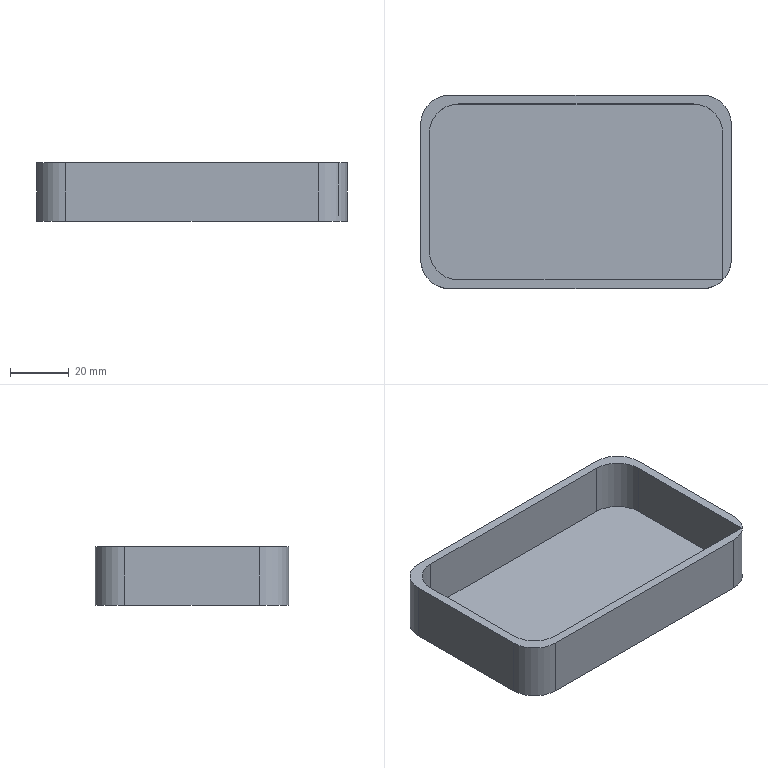Part | STEP file | 1 solid | 18 faces | box 106 x 66 x 20 mm | volume 31362 mm3 | plane 11 | cylinder 7 | commonest cylinder face diameters 20 x7
STEP:
#1=CARTESIAN_POINT('',(0.,0.,0.));
#2=DIRECTION('',(0.,0.,1.));
#3=DIRECTION('',(1.,0.,0.));
#4=AXIS2_PLACEMENT_3D('',#1,#2,#3);
#5=CARTESIAN_POINT('',(44.495,34.063,0.));
#6=VERTEX_POINT('',#5);
#7=CARTESIAN_POINT('',(-41.505,34.063,0.));
#8=VERTEX_POINT('',#7);
#9=CARTESIAN_POINT('',(1.495,34.063,0.));
#10=DIRECTION('',(-1.,0.,0.));
#11=VECTOR('',#10,1.);
#12=LINE('',#9,#11);
#13=CARTESIAN_POINT('',(1.495,1.063,0.));
#14=DIRECTION('',(0.,0.,1.));
#15=DIRECTION('',(1.,0.,0.));
#16=AXIS2_PLACEMENT_3D('',#13,#14,#15);
#17=PLANE('',#16);
#18=CARTESIAN_POINT('',(0.,33.));
#19=DIRECTION('',(-1.,0.));
#20=VECTOR('',#19,1.);
#21=LINE('',#18,#20);
#22=(GEOMETRIC_REPRESENTATION_CONTEXT(2)PARAMETRIC_REPRESENTATION_CONTEXT()REPRESENTATION_CONTEXT('',''));
#23=DEFINITIONAL_REPRESENTATION('',(#21),#22);
#24=PCURVE('',#17,#23);
#25=CARTESIAN_POINT('',(54.495,34.063,0.));
#26=DIRECTION('',(0.,1.,0.));
#27=DIRECTION('',(-1.,0.,0.));
#28=AXIS2_PLACEMENT_3D('',#25,#26,#27);
#29=PLANE('',#28);
#30=CARTESIAN_POINT('',(53.,0.));
#31=DIRECTION('',(1.,0.));
#32=VECTOR('',#31,1.);
#33=LINE('',#30,#32);
#34=(GEOMETRIC_REPRESENTATION_CONTEXT(2)PARAMETRIC_REPRESENTATION_CONTEXT()REPRESENTATION_CONTEXT('',''));
#35=DEFINITIONAL_REPRESENTATION('',(#33),#34);
#36=PCURVE('',#29,#35);
#37=SURFACE_CURVE('',#12,(#24,#36),.PCURVE_S1.);
#38=EDGE_CURVE('',#6,#8,#37,.T.);
#39=ORIENTED_EDGE('',*,*,#38,.F.);
#40=CARTESIAN_POINT('',(54.495,24.063,0.));
#41=VERTEX_POINT('',#40);
#42=CARTESIAN_POINT('',(44.495,24.063,0.));
#43=DIRECTION('',(0.,0.,1.));
#44=DIRECTION('',(1.,0.,0.));
#45=AXIS2_PLACEMENT_3D('',#42,#43,#44);
#46=CIRCLE('',#45,10.);
#47=CARTESIAN_POINT('',(43.,23.));
#48=DIRECTION('',(1.,0.));
#49=AXIS2_PLACEMENT_2D('',#47,#48);
#50=CIRCLE('',#49,10.);
#51=(GEOMETRIC_REPRESENTATION_CONTEXT(2)PARAMETRIC_REPRESENTATION_CONTEXT()REPRESENTATION_CONTEXT('',''));
#52=DEFINITIONAL_REPRESENTATION('',(#50),#51);
#53=PCURVE('',#17,#52);
#54=CARTESIAN_POINT('',(44.495,24.063,0.));
#55=DIRECTION('',(0.,0.,1.));
#56=DIRECTION('',(1.,0.,0.));
#57=AXIS2_PLACEMENT_3D('',#54,#55,#56);
#58=CYLINDRICAL_SURFACE('',#57,10.);
#59=CARTESIAN_POINT('',(0.,0.));
#60=DIRECTION('',(1.,0.));
#61=VECTOR('',#60,1.);
#62=LINE('',#59,#61);
#63=(GEOMETRIC_REPRESENTATION_CONTEXT(2)PARAMETRIC_REPRESENTATION_CONTEXT()REPRESENTATION_CONTEXT('',''));
#64=DEFINITIONAL_REPRESENTATION('',(#62),#63);
#65=PCURVE('',#58,#64);
#66=SURFACE_CURVE('',#46,(#53,#65),.PCURVE_S1.);
#67=EDGE_CURVE('',#41,#6,#66,.T.);
#68=ORIENTED_EDGE('',*,*,#67,.F.);
#69=CARTESIAN_POINT('',(54.495,-21.937,0.));
#70=VERTEX_POINT('',#69);
#71=CARTESIAN_POINT('',(54.495,1.063,0.));
#72=DIRECTION('',(0.,1.,0.));
#73=VECTOR('',#72,1.);
#74=LINE('',#71,#73);
#75=CARTESIAN_POINT('',(53.,0.));
#76=DIRECTION('',(0.,1.));
#77=VECTOR('',#76,1.);
#78=LINE('',#75,#77);
#79=(GEOMETRIC_REPRESENTATION_CONTEXT(2)PARAMETRIC_REPRESENTATION_CONTEXT()REPRESENTATION_CONTEXT('',''));
#80=DEFINITIONAL_REPRESENTATION('',(#78),#79);
#81=PCURVE('',#17,#80);
#82=CARTESIAN_POINT('',(54.495,-31.937,0.));
#83=DIRECTION('',(1.,0.,0.));
#84=DIRECTION('',(0.,1.,0.));
#85=AXIS2_PLACEMENT_3D('',#82,#83,#84);
#86=PLANE('',#85);
#87=CARTESIAN_POINT('',(33.,0.));
#88=DIRECTION('',(1.,0.));
#89=VECTOR('',#88,1.);
#90=LINE('',#87,#89);
#91=(GEOMETRIC_REPRESENTATION_CONTEXT(2)PARAMETRIC_REPRESENTATION_CONTEXT()REPRESENTATION_CONTEXT('',''));
#92=DEFINITIONAL_REPRESENTATION('',(#90),#91);
#93=PCURVE('',#86,#92);
#94=SURFACE_CURVE('',#74,(#81,#93),.PCURVE_S1.);
#95=EDGE_CURVE('',#70,#41,#94,.T.);
#96=ORIENTED_EDGE('',*,*,#95,.F.);
#97=CARTESIAN_POINT('',(44.495,-31.937,0.));
#98=VERTEX_POINT('',#97);
#99=CARTESIAN_POINT('',(44.495,-21.937,0.));
#100=DIRECTION('',(0.,0.,1.));
#101=DIRECTION('',(1.,0.,0.));
#102=AXIS2_PLACEMENT_3D('',#99,#100,#101);
#103=CIRCLE('',#102,10.);
#104=CARTESIAN_POINT('',(43.,-23.));
#105=DIRECTION('',(1.,0.));
#106=AXIS2_PLACEMENT_2D('',#104,#105);
#107=CIRCLE('',#106,10.);
#108=(GEOMETRIC_REPRESENTATION_CONTEXT(2)PARAMETRIC_REPRESENTATION_CONTEXT()REPRESENTATION_CONTEXT('',''));
#109=DEFINITIONAL_REPRESENTATION('',(#107),#108);
#110=PCURVE('',#17,#109);
#111=CARTESIAN_POINT('',(44.495,-21.937,0.));
#112=DIRECTION('',(0.,0.,1.));
#113=DIRECTION('',(1.,0.,0.));
#114=AXIS2_PLACEMENT_3D('',#111,#112,#113);
#115=CYLINDRICAL_SURFACE('',#114,10.);
#116=CARTESIAN_POINT('',(0.,0.));
#117=DIRECTION('',(1.,0.));
#118=VECTOR('',#117,1.);
#119=LINE('',#116,#118);
#120=(GEOMETRIC_REPRESENTATION_CONTEXT(2)PARAMETRIC_REPRESENTATION_CONTEXT()REPRESENTATION_CONTEXT('',''));
#121=DEFINITIONAL_REPRESENTATION('',(#119),#120);
#122=PCURVE('',#115,#121);
#123=SURFACE_CURVE('',#103,(#110,#122),.PCURVE_S1.);
#124=EDGE_CURVE('',#98,#70,#123,.T.);
#125=ORIENTED_EDGE('',*,*,#124,.F.);
#126=CARTESIAN_POINT('',(-41.505,-31.937,0.));
#127=VERTEX_POINT('',#126);
#128=CARTESIAN_POINT('',(1.495,-31.937,0.));
#129=DIRECTION('',(1.,0.,0.));
#130=VECTOR('',#129,1.);
#131=LINE('',#128,#130);
#132=CARTESIAN_POINT('',(0.,-33.));
#133=DIRECTION('',(1.,0.));
#134=VECTOR('',#133,1.);
#135=LINE('',#132,#134);
#136=(GEOMETRIC_REPRESENTATION_CONTEXT(2)PARAMETRIC_REPRESENTATION_CONTEXT()REPRESENTATION_CONTEXT('',''));
#137=DEFINITIONAL_REPRESENTATION('',(#135),#136);
#138=PCURVE('',#17,#137);
#139=CARTESIAN_POINT('',(-51.505,-31.937,0.));
#140=DIRECTION('',(0.,-1.,0.));
#141=DIRECTION('',(1.,0.,0.));
#142=AXIS2_PLACEMENT_3D('',#139,#140,#141);
#143=PLANE('',#142);
#144=CARTESIAN_POINT('',(53.,0.));
#145=DIRECTION('',(1.,0.));
#146=VECTOR('',#145,1.);
#147=LINE('',#144,#146);
#148=(GEOMETRIC_REPRESENTATION_CONTEXT(2)PARAMETRIC_REPRESENTATION_CONTEXT()REPRESENTATION_CONTEXT('',''));
#149=DEFINITIONAL_REPRESENTATION('',(#147),#148);
#150=PCURVE('',#143,#149);
#151=SURFACE_CURVE('',#131,(#138,#150),.PCURVE_S1.);
#152=EDGE_CURVE('',#127,#98,#151,.T.);
#153=ORIENTED_EDGE('',*,*,#152,.F.);
#154=CARTESIAN_POINT('',(-51.505,-21.937,0.));
#155=VERTEX_POINT('',#154);
#156=CARTESIAN_POINT('',(-41.505,-21.937,0.));
#157=DIRECTION('',(0.,0.,1.));
#158=DIRECTION('',(1.,0.,0.));
#159=AXIS2_PLACEMENT_3D('',#156,#157,#158);
#160=CIRCLE('',#159,10.);
#161=CARTESIAN_POINT('',(-43.,-23.));
#162=DIRECTION('',(1.,0.));
#163=AXIS2_PLACEMENT_2D('',#161,#162);
#164=CIRCLE('',#163,10.);
#165=(GEOMETRIC_REPRESENTATION_CONTEXT(2)PARAMETRIC_REPRESENTATION_CONTEXT()REPRESENTATION_CONTEXT('',''));
#166=DEFINITIONAL_REPRESENTATION('',(#164),#165);
#167=PCURVE('',#17,#166);
#168=CARTESIAN_POINT('',(-41.505,-21.937,0.));
#169=DIRECTION('',(0.,0.,1.));
#170=DIRECTION('',(1.,0.,0.));
#171=AXIS2_PLACEMENT_3D('',#168,#169,#170);
#172=CYLINDRICAL_SURFACE('',#171,10.);
#173=CARTESIAN_POINT('',(0.,0.));
#174=DIRECTION('',(1.,0.));
#175=VECTOR('',#174,1.);
#176=LINE('',#173,#175);
#177=(GEOMETRIC_REPRESENTATION_CONTEXT(2)PARAMETRIC_REPRESENTATION_CONTEXT()REPRESENTATION_CONTEXT('',''));
#178=DEFINITIONAL_REPRESENTATION('',(#176),#177);
#179=PCURVE('',#172,#178);
#180=SURFACE_CURVE('',#160,(#167,#179),.PCURVE_S1.);
#181=EDGE_CURVE('',#155,#127,#180,.T.);
#182=ORIENTED_EDGE('',*,*,#181,.F.);
#183=CARTESIAN_POINT('',(-51.505,24.063,0.));
#184=VERTEX_POINT('',#183);
#185=CARTESIAN_POINT('',(-51.505,1.063,0.));
#186=DIRECTION('',(0.,-1.,0.));
#187=VECTOR('',#186,1.);
#188=LINE('',#185,#187);
#189=CARTESIAN_POINT('',(-53.,0.));
#190=DIRECTION('',(0.,-1.));
#191=VECTOR('',#190,1.);
#192=LINE('',#189,#191);
#193=(GEOMETRIC_REPRESENTATION_CONTEXT(2)PARAMETRIC_REPRESENTATION_CONTEXT()REPRESENTATION_CONTEXT('',''));
#194=DEFINITIONAL_REPRESENTATION('',(#192),#193);
#195=PCURVE('',#17,#194);
#196=CARTESIAN_POINT('',(-51.505,34.063,0.));
#197=DIRECTION('',(-1.,0.,0.));
#198=DIRECTION('',(0.,-1.,0.));
#199=AXIS2_PLACEMENT_3D('',#196,#197,#198);
#200=PLANE('',#199);
#201=CARTESIAN_POINT('',(33.,0.));
#202=DIRECTION('',(1.,0.));
#203=VECTOR('',#202,1.);
#204=LINE('',#201,#203);
#205=(GEOMETRIC_REPRESENTATION_CONTEXT(2)PARAMETRIC_REPRESENTATION_CONTEXT()REPRESENTATION_CONTEXT('',''));
#206=DEFINITIONAL_REPRESENTATION('',(#204),#205);
#207=PCURVE('',#200,#206);
#208=SURFACE_CURVE('',#188,(#195,#207),.PCURVE_S1.);
#209=EDGE_CURVE('',#184,#155,#208,.T.);
#210=ORIENTED_EDGE('',*,*,#209,.F.);
#211=CARTESIAN_POINT('',(-41.505,24.063,0.));
#212=DIRECTION('',(0.,0.,1.));
#213=DIRECTION('',(1.,0.,0.));
#214=AXIS2_PLACEMENT_3D('',#211,#212,#213);
#215=CIRCLE('',#214,10.);
#216=CARTESIAN_POINT('',(-43.,23.));
#217=DIRECTION('',(1.,0.));
#218=AXIS2_PLACEMENT_2D('',#216,#217);
#219=CIRCLE('',#218,10.);
#220=(GEOMETRIC_REPRESENTATION_CONTEXT(2)PARAMETRIC_REPRESENTATION_CONTEXT()REPRESENTATION_CONTEXT('',''));
#221=DEFINITIONAL_REPRESENTATION('',(#219),#220);
#222=PCURVE('',#17,#221);
#223=CARTESIAN_POINT('',(-41.505,24.063,0.));
#224=DIRECTION('',(0.,0.,1.));
#225=DIRECTION('',(1.,0.,0.));
#226=AXIS2_PLACEMENT_3D('',#223,#224,#225);
#227=CYLINDRICAL_SURFACE('',#226,10.);
#228=CARTESIAN_POINT('',(0.,0.));
#229=DIRECTION('',(1.,0.));
#230=VECTOR('',#229,1.);
#231=LINE('',#228,#230);
#232=(GEOMETRIC_REPRESENTATION_CONTEXT(2)PARAMETRIC_REPRESENTATION_CONTEXT()REPRESENTATION_CONTEXT('',''));
#233=DEFINITIONAL_REPRESENTATION('',(#231),#232);
#234=PCURVE('',#227,#233);
#235=SURFACE_CURVE('',#215,(#222,#234),.PCURVE_S1.);
#236=EDGE_CURVE('',#8,#184,#235,.T.);
#237=ORIENTED_EDGE('',*,*,#236,.F.);
#238=EDGE_LOOP('',(#39,#68,#96,#125,#153,#182,#210,#237));
#239=FACE_BOUND('',#238,.T.);
#240=ADVANCED_FACE('',(#239),#17,.F.);
#241=ORIENTED_EDGE('',*,*,#236,.T.);
#242=CARTESIAN_POINT('',(-51.505,24.063,20.));
#243=VERTEX_POINT('',#242);
#244=CARTESIAN_POINT('',(-51.505,24.063,0.));
#245=DIRECTION('',(0.,0.,1.));
#246=VECTOR('',#245,1.);
#247=LINE('',#244,#246);
#248=CARTESIAN_POINT('',(3.142,0.));
#249=DIRECTION('',(0.,1.));
#250=VECTOR('',#249,1.);
#251=LINE('',#248,#250);
#252=(GEOMETRIC_REPRESENTATION_CONTEXT(2)PARAMETRIC_REPRESENTATION_CONTEXT()REPRESENTATION_CONTEXT('',''));
#253=DEFINITIONAL_REPRESENTATION('',(#251),#252);
#254=PCURVE('',#227,#253);
#255=CARTESIAN_POINT('',(10.,0.));
#256=DIRECTION('',(0.,1.));
#257=VECTOR('',#256,1.);
#258=LINE('',#255,#257);
#259=(GEOMETRIC_REPRESENTATION_CONTEXT(2)PARAMETRIC_REPRESENTATION_CONTEXT()REPRESENTATION_CONTEXT('',''));
#260=DEFINITIONAL_REPRESENTATION('',(#258),#259);
#261=PCURVE('',#200,#260);
#262=SURFACE_CURVE('',#247,(#254,#261),.PCURVE_S1.);
#263=EDGE_CURVE('',#184,#243,#262,.T.);
#264=ORIENTED_EDGE('',*,*,#263,.T.);
#265=CARTESIAN_POINT('',(-41.505,34.063,20.));
#266=VERTEX_POINT('',#265);
#267=CARTESIAN_POINT('',(-41.505,24.063,20.));
#268=DIRECTION('',(0.,0.,-1.));
#269=DIRECTION('',(1.,0.,0.));
#270=AXIS2_PLACEMENT_3D('',#267,#268,#269);
#271=CIRCLE('',#270,10.);
#272=CARTESIAN_POINT('',(6.283,20.));
#273=DIRECTION('',(-1.,0.));
#274=VECTOR('',#273,1.);
#275=LINE('',#272,#274);
#276=(GEOMETRIC_REPRESENTATION_CONTEXT(2)PARAMETRIC_REPRESENTATION_CONTEXT()REPRESENTATION_CONTEXT('',''));
#277=DEFINITIONAL_REPRESENTATION('',(#275),#276);
#278=PCURVE('',#227,#277);
#279=CARTESIAN_POINT('',(1.495,1.063,20.));
#280=DIRECTION('',(0.,0.,1.));
#281=DIRECTION('',(1.,0.,0.));
#282=AXIS2_PLACEMENT_3D('',#279,#280,#281);
#283=PLANE('',#282);
#284=CARTESIAN_POINT('',(-33.,23.));
#285=CARTESIAN_POINT('',(-33.,5.679));
#286=CARTESIAN_POINT('',(-48.,14.34));
#287=CARTESIAN_POINT('',(-63.,23.));
#288=CARTESIAN_POINT('',(-48.,31.66));
#289=CARTESIAN_POINT('',(-33.,40.321));
#290=CARTESIAN_POINT('',(-33.,23.));
#291=(BOUNDED_CURVE()B_SPLINE_CURVE(2,(#284,#285,#286,#287,#288,#289,#290),.UNSPECIFIED.,.T.,.F.)B_SPLINE_CURVE_WITH_KNOTS((1,2,2,2,2,1),(-2.094,0.,2.094,4.189,6.283,8.378),.UNSPECIFIED.)CURVE()GEOMETRIC_REPRESENTATION_ITEM()RATIONAL_B_SPLINE_CURVE((1.,0.5,1.,0.5,1.,0.5,1.))REPRESENTATION_ITEM(''));
#292=(GEOMETRIC_REPRESENTATION_CONTEXT(2)PARAMETRIC_REPRESENTATION_CONTEXT()REPRESENTATION_CONTEXT('',''));
#293=DEFINITIONAL_REPRESENTATION('',(#291),#292);
#294=PCURVE('',#283,#293);
#295=SURFACE_CURVE('',#271,(#278,#294),.PCURVE_S1.);
#296=EDGE_CURVE('',#243,#266,#295,.T.);
#297=ORIENTED_EDGE('',*,*,#296,.T.);
#298=CARTESIAN_POINT('',(-41.505,34.063,0.));
#299=DIRECTION('',(0.,0.,-1.));
#300=VECTOR('',#299,1.);
#301=LINE('',#298,#300);
#302=CARTESIAN_POINT('',(1.571,0.));
#303=DIRECTION('',(0.,-1.));
#304=VECTOR('',#303,1.);
#305=LINE('',#302,#304);
#306=(GEOMETRIC_REPRESENTATION_CONTEXT(2)PARAMETRIC_REPRESENTATION_CONTEXT()REPRESENTATION_CONTEXT('',''));
#307=DEFINITIONAL_REPRESENTATION('',(#305),#306);
#308=PCURVE('',#227,#307);
#309=CARTESIAN_POINT('',(96.,0.));
#310=DIRECTION('',(0.,-1.));
#311=VECTOR('',#310,1.);
#312=LINE('',#309,#311);
#313=(GEOMETRIC_REPRESENTATION_CONTEXT(2)PARAMETRIC_REPRESENTATION_CONTEXT()REPRESENTATION_CONTEXT('',''));
#314=DEFINITIONAL_REPRESENTATION('',(#312),#313);
#315=PCURVE('',#29,#314);
#316=SURFACE_CURVE('',#301,(#308,#315),.PCURVE_S1.);
#317=EDGE_CURVE('',#266,#8,#316,.T.);
#318=ORIENTED_EDGE('',*,*,#317,.T.);
#319=EDGE_LOOP('',(#241,#264,#297,#318));
#320=FACE_BOUND('',#319,.T.);
#321=ADVANCED_FACE('',(#320),#227,.T.);
#322=CARTESIAN_POINT('',(44.495,34.063,20.));
#323=VERTEX_POINT('',#322);
#324=CARTESIAN_POINT('',(44.495,34.063,0.));
#325=DIRECTION('',(0.,0.,-1.));
#326=VECTOR('',#325,1.);
#327=LINE('',#324,#326);
#328=CARTESIAN_POINT('',(10.,0.));
#329=DIRECTION('',(0.,-1.));
#330=VECTOR('',#329,1.);
#331=LINE('',#328,#330);
#332=(GEOMETRIC_REPRESENTATION_CONTEXT(2)PARAMETRIC_REPRESENTATION_CONTEXT()REPRESENTATION_CONTEXT('',''));
#333=DEFINITIONAL_REPRESENTATION('',(#331),#332);
#334=PCURVE('',#29,#333);
#335=CARTESIAN_POINT('',(1.571,0.));
#336=DIRECTION('',(0.,-1.));
#337=VECTOR('',#336,1.);
#338=LINE('',#335,#337);
#339=(GEOMETRIC_REPRESENTATION_CONTEXT(2)PARAMETRIC_REPRESENTATION_CONTEXT()REPRESENTATION_CONTEXT('',''));
#340=DEFINITIONAL_REPRESENTATION('',(#338),#339);
#341=PCURVE('',#58,#340);
#342=SURFACE_CURVE('',#327,(#334,#341),.PCURVE_S1.);
#343=EDGE_CURVE('',#323,#6,#342,.T.);
#344=ORIENTED_EDGE('',*,*,#343,.T.);
#345=ORIENTED_EDGE('',*,*,#38,.T.);
#346=ORIENTED_EDGE('',*,*,#317,.F.);
#347=CARTESIAN_POINT('',(54.495,34.063,20.));
#348=DIRECTION('',(1.,0.,0.));
#349=VECTOR('',#348,1.);
#350=LINE('',#347,#349);
#351=CARTESIAN_POINT('',(0.,20.));
#352=DIRECTION('',(-1.,0.));
#353=VECTOR('',#352,1.);
#354=LINE('',#351,#353);
#355=(GEOMETRIC_REPRESENTATION_CONTEXT(2)PARAMETRIC_REPRESENTATION_CONTEXT()REPRESENTATION_CONTEXT('',''));
#356=DEFINITIONAL_REPRESENTATION('',(#354),#355);
#357=PCURVE('',#29,#356);
#358=CARTESIAN_POINT('',(53.,33.));
#359=DIRECTION('',(1.,0.));
#360=VECTOR('',#359,1.);
#361=LINE('',#358,#360);
#362=(GEOMETRIC_REPRESENTATION_CONTEXT(2)PARAMETRIC_REPRESENTATION_CONTEXT()REPRESENTATION_CONTEXT('',''));
#363=DEFINITIONAL_REPRESENTATION('',(#361),#362);
#364=PCURVE('',#283,#363);
#365=SURFACE_CURVE('',#350,(#357,#364),.PCURVE_S1.);
#366=EDGE_CURVE('',#266,#323,#365,.T.);
#367=ORIENTED_EDGE('',*,*,#366,.T.);
#368=EDGE_LOOP('',(#344,#345,#346,#367));
#369=FACE_BOUND('',#368,.T.);
#370=ADVANCED_FACE('',(#369),#29,.T.);
#371=ORIENTED_EDGE('',*,*,#67,.T.);
#372=ORIENTED_EDGE('',*,*,#343,.F.);
#373=CARTESIAN_POINT('',(54.495,24.063,20.));
#374=VERTEX_POINT('',#373);
#375=CARTESIAN_POINT('',(44.495,24.063,20.));
#376=DIRECTION('',(0.,0.,-1.));
#377=DIRECTION('',(1.,0.,0.));
#378=AXIS2_PLACEMENT_3D('',#375,#376,#377);
#379=CIRCLE('',#378,10.);
#380=CARTESIAN_POINT('',(6.283,20.));
#381=DIRECTION('',(-1.,0.));
#382=VECTOR('',#381,1.);
#383=LINE('',#380,#382);
#384=(GEOMETRIC_REPRESENTATION_CONTEXT(2)PARAMETRIC_REPRESENTATION_CONTEXT()REPRESENTATION_CONTEXT('',''));
#385=DEFINITIONAL_REPRESENTATION('',(#383),#384);
#386=PCURVE('',#58,#385);
#387=CARTESIAN_POINT('',(53.,23.));
#388=CARTESIAN_POINT('',(53.,5.679));
#389=CARTESIAN_POINT('',(38.,14.34));
#390=CARTESIAN_POINT('',(23.,23.));
#391=CARTESIAN_POINT('',(38.,31.66));
#392=CARTESIAN_POINT('',(53.,40.321));
#393=CARTESIAN_POINT('',(53.,23.));
#394=(BOUNDED_CURVE()B_SPLINE_CURVE(2,(#387,#388,#389,#390,#391,#392,#393),.UNSPECIFIED.,.T.,.F.)B_SPLINE_CURVE_WITH_KNOTS((1,2,2,2,2,1),(-2.094,0.,2.094,4.189,6.283,8.378),.UNSPECIFIED.)CURVE()GEOMETRIC_REPRESENTATION_ITEM()RATIONAL_B_SPLINE_CURVE((1.,0.5,1.,0.5,1.,0.5,1.))REPRESENTATION_ITEM(''));
#395=(GEOMETRIC_REPRESENTATION_CONTEXT(2)PARAMETRIC_REPRESENTATION_CONTEXT()REPRESENTATION_CONTEXT('',''));
#396=DEFINITIONAL_REPRESENTATION('',(#394),#395);
#397=PCURVE('',#283,#396);
#398=SURFACE_CURVE('',#379,(#386,#397),.PCURVE_S1.);
#399=EDGE_CURVE('',#323,#374,#398,.T.);
#400=ORIENTED_EDGE('',*,*,#399,.T.);
#401=CARTESIAN_POINT('',(54.495,24.063,0.));
#402=DIRECTION('',(0.,0.,-1.));
#403=VECTOR('',#402,1.);
#404=LINE('',#401,#403);
#405=CARTESIAN_POINT('',(0.,0.));
#406=DIRECTION('',(0.,-1.));
#407=VECTOR('',#406,1.);
#408=LINE('',#405,#407);
#409=(GEOMETRIC_REPRESENTATION_CONTEXT(2)PARAMETRIC_REPRESENTATION_CONTEXT()REPRESENTATION_CONTEXT('',''));
#410=DEFINITIONAL_REPRESENTATION('',(#408),#409);
#411=PCURVE('',#58,#410);
#412=CARTESIAN_POINT('',(56.,0.));
#413=DIRECTION('',(0.,-1.));
#414=VECTOR('',#413,1.);
#415=LINE('',#412,#414);
#416=(GEOMETRIC_REPRESENTATION_CONTEXT(2)PARAMETRIC_REPRESENTATION_CONTEXT()REPRESENTATION_CONTEXT('',''));
#417=DEFINITIONAL_REPRESENTATION('',(#415),#416);
#418=PCURVE('',#86,#417);
#419=SURFACE_CURVE('',#404,(#411,#418),.PCURVE_S1.);
#420=EDGE_CURVE('',#374,#41,#419,.T.);
#421=ORIENTED_EDGE('',*,*,#420,.T.);
#422=EDGE_LOOP('',(#371,#372,#400,#421));
#423=FACE_BOUND('',#422,.T.);
#424=ADVANCED_FACE('',(#423),#58,.T.);
#425=CARTESIAN_POINT('',(54.495,-21.937,20.));
#426=VERTEX_POINT('',#425);
#427=CARTESIAN_POINT('',(54.495,-21.937,0.));
#428=DIRECTION('',(0.,0.,-1.));
#429=VECTOR('',#428,1.);
#430=LINE('',#427,#429);
#431=CARTESIAN_POINT('',(10.,0.));
#432=DIRECTION('',(0.,-1.));
#433=VECTOR('',#432,1.);
#434=LINE('',#431,#433);
#435=(GEOMETRIC_REPRESENTATION_CONTEXT(2)PARAMETRIC_REPRESENTATION_CONTEXT()REPRESENTATION_CONTEXT('',''));
#436=DEFINITIONAL_REPRESENTATION('',(#434),#435);
#437=PCURVE('',#86,#436);
#438=CARTESIAN_POINT('',(6.283,0.));
#439=DIRECTION('',(0.,-1.));
#440=VECTOR('',#439,1.);
#441=LINE('',#438,#440);
#442=(GEOMETRIC_REPRESENTATION_CONTEXT(2)PARAMETRIC_REPRESENTATION_CONTEXT()REPRESENTATION_CONTEXT('',''));
#443=DEFINITIONAL_REPRESENTATION('',(#441),#442);
#444=PCURVE('',#115,#443);
#445=SURFACE_CURVE('',#430,(#437,#444),.PCURVE_S1.);
#446=EDGE_CURVE('',#426,#70,#445,.T.);
#447=ORIENTED_EDGE('',*,*,#446,.T.);
#448=ORIENTED_EDGE('',*,*,#95,.T.);
#449=ORIENTED_EDGE('',*,*,#420,.F.);
#450=CARTESIAN_POINT('',(54.495,-31.937,20.));
#451=DIRECTION('',(0.,-1.,0.));
#452=VECTOR('',#451,1.);
#453=LINE('',#450,#452);
#454=CARTESIAN_POINT('',(0.,20.));
#455=DIRECTION('',(-1.,0.));
#456=VECTOR('',#455,1.);
#457=LINE('',#454,#456);
#458=(GEOMETRIC_REPRESENTATION_CONTEXT(2)PARAMETRIC_REPRESENTATION_CONTEXT()REPRESENTATION_CONTEXT('',''));
#459=DEFINITIONAL_REPRESENTATION('',(#457),#458);
#460=PCURVE('',#86,#459);
#461=CARTESIAN_POINT('',(53.,-33.));
#462=DIRECTION('',(0.,-1.));
#463=VECTOR('',#462,1.);
#464=LINE('',#461,#463);
#465=(GEOMETRIC_REPRESENTATION_CONTEXT(2)PARAMETRIC_REPRESENTATION_CONTEXT()REPRESENTATION_CONTEXT('',''));
#466=DEFINITIONAL_REPRESENTATION('',(#464),#465);
#467=PCURVE('',#283,#466);
#468=SURFACE_CURVE('',#453,(#460,#467),.PCURVE_S1.);
#469=EDGE_CURVE('',#374,#426,#468,.T.);
#470=ORIENTED_EDGE('',*,*,#469,.T.);
#471=EDGE_LOOP('',(#447,#448,#449,#470));
#472=FACE_BOUND('',#471,.T.);
#473=ADVANCED_FACE('',(#472),#86,.T.);
#474=ORIENTED_EDGE('',*,*,#124,.T.);
#475=ORIENTED_EDGE('',*,*,#446,.F.);
#476=CARTESIAN_POINT('',(44.495,-31.937,20.));
#477=VERTEX_POINT('',#476);
#478=CARTESIAN_POINT('',(44.495,-21.937,20.));
#479=DIRECTION('',(0.,0.,-1.));
#480=DIRECTION('',(1.,0.,0.));
#481=AXIS2_PLACEMENT_3D('',#478,#479,#480);
#482=CIRCLE('',#481,10.);
#483=CARTESIAN_POINT('',(6.283,20.));
#484=DIRECTION('',(-1.,0.));
#485=VECTOR('',#484,1.);
#486=LINE('',#483,#485);
#487=(GEOMETRIC_REPRESENTATION_CONTEXT(2)PARAMETRIC_REPRESENTATION_CONTEXT()REPRESENTATION_CONTEXT('',''));
#488=DEFINITIONAL_REPRESENTATION('',(#486),#487);
#489=PCURVE('',#115,#488);
#490=CARTESIAN_POINT('',(53.,-23.));
#491=CARTESIAN_POINT('',(53.,-40.321));
#492=CARTESIAN_POINT('',(38.,-31.66));
#493=CARTESIAN_POINT('',(23.,-23.));
#494=CARTESIAN_POINT('',(38.,-14.34));
#495=CARTESIAN_POINT('',(53.,-5.679));
#496=CARTESIAN_POINT('',(53.,-23.));
#497=(BOUNDED_CURVE()B_SPLINE_CURVE(2,(#490,#491,#492,#493,#494,#495,#496),.UNSPECIFIED.,.T.,.F.)B_SPLINE_CURVE_WITH_KNOTS((1,2,2,2,2,1),(-2.094,0.,2.094,4.189,6.283,8.378),.UNSPECIFIED.)CURVE()GEOMETRIC_REPRESENTATION_ITEM()RATIONAL_B_SPLINE_CURVE((1.,0.5,1.,0.5,1.,0.5,1.))REPRESENTATION_ITEM(''));
#498=(GEOMETRIC_REPRESENTATION_CONTEXT(2)PARAMETRIC_REPRESENTATION_CONTEXT()REPRESENTATION_CONTEXT('',''));
#499=DEFINITIONAL_REPRESENTATION('',(#497),#498);
#500=PCURVE('',#283,#499);
#501=SURFACE_CURVE('',#482,(#489,#500),.PCURVE_S1.);
#502=EDGE_CURVE('',#426,#477,#501,.T.);
#503=ORIENTED_EDGE('',*,*,#502,.T.);
#504=CARTESIAN_POINT('',(44.495,-31.937,0.));
#505=DIRECTION('',(0.,0.,-1.));
#506=VECTOR('',#505,1.);
#507=LINE('',#504,#506);
#508=CARTESIAN_POINT('',(4.712,0.));
#509=DIRECTION('',(0.,-1.));
#510=VECTOR('',#509,1.);
#511=LINE('',#508,#510);
#512=(GEOMETRIC_REPRESENTATION_CONTEXT(2)PARAMETRIC_REPRESENTATION_CONTEXT()REPRESENTATION_CONTEXT('',''));
#513=DEFINITIONAL_REPRESENTATION('',(#511),#512);
#514=PCURVE('',#115,#513);
#515=CARTESIAN_POINT('',(96.,0.));
#516=DIRECTION('',(0.,-1.));
#517=VECTOR('',#516,1.);
#518=LINE('',#515,#517);
#519=(GEOMETRIC_REPRESENTATION_CONTEXT(2)PARAMETRIC_REPRESENTATION_CONTEXT()REPRESENTATION_CONTEXT('',''));
#520=DEFINITIONAL_REPRESENTATION('',(#518),#519);
#521=PCURVE('',#143,#520);
#522=SURFACE_CURVE('',#507,(#514,#521),.PCURVE_S1.);
#523=EDGE_CURVE('',#477,#98,#522,.T.);
#524=ORIENTED_EDGE('',*,*,#523,.T.);
#525=EDGE_LOOP('',(#474,#475,#503,#524));
#526=FACE_BOUND('',#525,.T.);
#527=ADVANCED_FACE('',(#526),#115,.T.);
#528=CARTESIAN_POINT('',(-41.505,-31.937,20.));
#529=VERTEX_POINT('',#528);
#530=CARTESIAN_POINT('',(-41.505,-31.937,0.));
#531=DIRECTION('',(0.,0.,-1.));
#532=VECTOR('',#531,1.);
#533=LINE('',#530,#532);
#534=CARTESIAN_POINT('',(10.,0.));
#535=DIRECTION('',(0.,-1.));
#536=VECTOR('',#535,1.);
#537=LINE('',#534,#536);
#538=(GEOMETRIC_REPRESENTATION_CONTEXT(2)PARAMETRIC_REPRESENTATION_CONTEXT()REPRESENTATION_CONTEXT('',''));
#539=DEFINITIONAL_REPRESENTATION('',(#537),#538);
#540=PCURVE('',#143,#539);
#541=CARTESIAN_POINT('',(4.712,0.));
#542=DIRECTION('',(0.,-1.));
#543=VECTOR('',#542,1.);
#544=LINE('',#541,#543);
#545=(GEOMETRIC_REPRESENTATION_CONTEXT(2)PARAMETRIC_REPRESENTATION_CONTEXT()REPRESENTATION_CONTEXT('',''));
#546=DEFINITIONAL_REPRESENTATION('',(#544),#545);
#547=PCURVE('',#172,#546);
#548=SURFACE_CURVE('',#533,(#540,#547),.PCURVE_S1.);
#549=EDGE_CURVE('',#529,#127,#548,.T.);
#550=ORIENTED_EDGE('',*,*,#549,.T.);
#551=ORIENTED_EDGE('',*,*,#152,.T.);
#552=ORIENTED_EDGE('',*,*,#523,.F.);
#553=CARTESIAN_POINT('',(-51.505,-31.937,20.));
#554=DIRECTION('',(-1.,0.,0.));
#555=VECTOR('',#554,1.);
#556=LINE('',#553,#555);
#557=CARTESIAN_POINT('',(0.,20.));
#558=DIRECTION('',(-1.,0.));
#559=VECTOR('',#558,1.);
#560=LINE('',#557,#559);
#561=(GEOMETRIC_REPRESENTATION_CONTEXT(2)PARAMETRIC_REPRESENTATION_CONTEXT()REPRESENTATION_CONTEXT('',''));
#562=DEFINITIONAL_REPRESENTATION('',(#560),#561);
#563=PCURVE('',#143,#562);
#564=CARTESIAN_POINT('',(-53.,-33.));
#565=DIRECTION('',(-1.,0.));
#566=VECTOR('',#565,1.);
#567=LINE('',#564,#566);
#568=(GEOMETRIC_REPRESENTATION_CONTEXT(2)PARAMETRIC_REPRESENTATION_CONTEXT()REPRESENTATION_CONTEXT('',''));
#569=DEFINITIONAL_REPRESENTATION('',(#567),#568);
#570=PCURVE('',#283,#569);
#571=SURFACE_CURVE('',#556,(#563,#570),.PCURVE_S1.);
#572=EDGE_CURVE('',#477,#529,#571,.T.);
#573=ORIENTED_EDGE('',*,*,#572,.T.);
#574=EDGE_LOOP('',(#550,#551,#552,#573));
#575=FACE_BOUND('',#574,.T.);
#576=ADVANCED_FACE('',(#575),#143,.T.);
#577=ORIENTED_EDGE('',*,*,#181,.T.);
#578=ORIENTED_EDGE('',*,*,#549,.F.);
#579=CARTESIAN_POINT('',(-51.505,-21.937,20.));
#580=VERTEX_POINT('',#579);
#581=CARTESIAN_POINT('',(-41.505,-21.937,20.));
#582=DIRECTION('',(0.,0.,-1.));
#583=DIRECTION('',(1.,0.,0.));
#584=AXIS2_PLACEMENT_3D('',#581,#582,#583);
#585=CIRCLE('',#584,10.);
#586=CARTESIAN_POINT('',(6.283,20.));
#587=DIRECTION('',(-1.,0.));
#588=VECTOR('',#587,1.);
#589=LINE('',#586,#588);
#590=(GEOMETRIC_REPRESENTATION_CONTEXT(2)PARAMETRIC_REPRESENTATION_CONTEXT()REPRESENTATION_CONTEXT('',''));
#591=DEFINITIONAL_REPRESENTATION('',(#589),#590);
#592=PCURVE('',#172,#591);
#593=CARTESIAN_POINT('',(-33.,-23.));
#594=CARTESIAN_POINT('',(-33.,-40.321));
#595=CARTESIAN_POINT('',(-48.,-31.66));
#596=CARTESIAN_POINT('',(-63.,-23.));
#597=CARTESIAN_POINT('',(-48.,-14.34));
#598=CARTESIAN_POINT('',(-33.,-5.679));
#599=CARTESIAN_POINT('',(-33.,-23.));
#600=(BOUNDED_CURVE()B_SPLINE_CURVE(2,(#593,#594,#595,#596,#597,#598,#599),.UNSPECIFIED.,.T.,.F.)B_SPLINE_CURVE_WITH_KNOTS((1,2,2,2,2,1),(-2.094,0.,2.094,4.189,6.283,8.378),.UNSPECIFIED.)CURVE()GEOMETRIC_REPRESENTATION_ITEM()RATIONAL_B_SPLINE_CURVE((1.,0.5,1.,0.5,1.,0.5,1.))REPRESENTATION_ITEM(''));
#601=(GEOMETRIC_REPRESENTATION_CONTEXT(2)PARAMETRIC_REPRESENTATION_CONTEXT()REPRESENTATION_CONTEXT('',''));
#602=DEFINITIONAL_REPRESENTATION('',(#600),#601);
#603=PCURVE('',#283,#602);
#604=SURFACE_CURVE('',#585,(#592,#603),.PCURVE_S1.);
#605=EDGE_CURVE('',#529,#580,#604,.T.);
#606=ORIENTED_EDGE('',*,*,#605,.T.);
#607=CARTESIAN_POINT('',(-51.505,-21.937,0.));
#608=DIRECTION('',(0.,0.,-1.));
#609=VECTOR('',#608,1.);
#610=LINE('',#607,#609);
#611=CARTESIAN_POINT('',(3.142,0.));
#612=DIRECTION('',(0.,-1.));
#613=VECTOR('',#612,1.);
#614=LINE('',#611,#613);
#615=(GEOMETRIC_REPRESENTATION_CONTEXT(2)PARAMETRIC_REPRESENTATION_CONTEXT()REPRESENTATION_CONTEXT('',''));
#616=DEFINITIONAL_REPRESENTATION('',(#614),#615);
#617=PCURVE('',#172,#616);
#618=CARTESIAN_POINT('',(56.,0.));
#619=DIRECTION('',(0.,-1.));
#620=VECTOR('',#619,1.);
#621=LINE('',#618,#620);
#622=(GEOMETRIC_REPRESENTATION_CONTEXT(2)PARAMETRIC_REPRESENTATION_CONTEXT()REPRESENTATION_CONTEXT('',''));
#623=DEFINITIONAL_REPRESENTATION('',(#621),#622);
#624=PCURVE('',#200,#623);
#625=SURFACE_CURVE('',#610,(#617,#624),.PCURVE_S1.);
#626=EDGE_CURVE('',#580,#155,#625,.T.);
#627=ORIENTED_EDGE('',*,*,#626,.T.);
#628=EDGE_LOOP('',(#577,#578,#606,#627));
#629=FACE_BOUND('',#628,.T.);
#630=ADVANCED_FACE('',(#629),#172,.T.);
#631=ORIENTED_EDGE('',*,*,#626,.F.);
#632=CARTESIAN_POINT('',(-51.505,34.063,20.));
#633=DIRECTION('',(0.,1.,0.));
#634=VECTOR('',#633,1.);
#635=LINE('',#632,#634);
#636=CARTESIAN_POINT('',(0.,20.));
#637=DIRECTION('',(-1.,0.));
#638=VECTOR('',#637,1.);
#639=LINE('',#636,#638);
#640=(GEOMETRIC_REPRESENTATION_CONTEXT(2)PARAMETRIC_REPRESENTATION_CONTEXT()REPRESENTATION_CONTEXT('',''));
#641=DEFINITIONAL_REPRESENTATION('',(#639),#640);
#642=PCURVE('',#200,#641);
#643=CARTESIAN_POINT('',(-53.,33.));
#644=DIRECTION('',(0.,1.));
#645=VECTOR('',#644,1.);
#646=LINE('',#643,#645);
#647=(GEOMETRIC_REPRESENTATION_CONTEXT(2)PARAMETRIC_REPRESENTATION_CONTEXT()REPRESENTATION_CONTEXT('',''));
#648=DEFINITIONAL_REPRESENTATION('',(#646),#647);
#649=PCURVE('',#283,#648);
#650=SURFACE_CURVE('',#635,(#642,#649),.PCURVE_S1.);
#651=EDGE_CURVE('',#580,#243,#650,.T.);
#652=ORIENTED_EDGE('',*,*,#651,.T.);
#653=ORIENTED_EDGE('',*,*,#263,.F.);
#654=ORIENTED_EDGE('',*,*,#209,.T.);
#655=EDGE_LOOP('',(#631,#652,#653,#654));
#656=FACE_BOUND('',#655,.T.);
#657=ADVANCED_FACE('',(#656),#200,.T.);
#658=CARTESIAN_POINT('',(-38.505,31.063,20.));
#659=VERTEX_POINT('',#658);
#660=CARTESIAN_POINT('',(41.495,31.063,20.));
#661=VERTEX_POINT('',#660);
#662=CARTESIAN_POINT('',(1.495,31.063,20.));
#663=DIRECTION('',(1.,0.,0.));
#664=VECTOR('',#663,1.);
#665=LINE('',#662,#664);
#666=CARTESIAN_POINT('',(0.,30.));
#667=DIRECTION('',(1.,0.));
#668=VECTOR('',#667,1.);
#669=LINE('',#666,#668);
#670=(GEOMETRIC_REPRESENTATION_CONTEXT(2)PARAMETRIC_REPRESENTATION_CONTEXT()REPRESENTATION_CONTEXT('',''));
#671=DEFINITIONAL_REPRESENTATION('',(#669),#670);
#672=PCURVE('',#283,#671);
#673=CARTESIAN_POINT('',(51.495,31.063,0.));
#674=DIRECTION('',(0.,1.,0.));
#675=DIRECTION('',(0.,0.,1.));
#676=AXIS2_PLACEMENT_3D('',#673,#674,#675);
#677=PLANE('',#676);
#678=CARTESIAN_POINT('',(20.,-50.));
#679=DIRECTION('',(0.,1.));
#680=VECTOR('',#679,1.);
#681=LINE('',#678,#680);
#682=(GEOMETRIC_REPRESENTATION_CONTEXT(2)PARAMETRIC_REPRESENTATION_CONTEXT()REPRESENTATION_CONTEXT('',''));
#683=DEFINITIONAL_REPRESENTATION('',(#681),#682);
#684=PCURVE('',#677,#683);
#685=SURFACE_CURVE('',#665,(#672,#684),.PCURVE_S1.);
#686=EDGE_CURVE('',#659,#661,#685,.T.);
#687=ORIENTED_EDGE('',*,*,#686,.T.);
#688=CARTESIAN_POINT('',(51.495,21.063,20.));
#689=VERTEX_POINT('',#688);
#690=CARTESIAN_POINT('',(41.495,21.063,20.));
#691=DIRECTION('',(0.,0.,-1.));
#692=DIRECTION('',(1.,0.,0.));
#693=AXIS2_PLACEMENT_3D('',#690,#691,#692);
#694=CIRCLE('',#693,10.);
#695=CARTESIAN_POINT('',(50.,20.));
#696=CARTESIAN_POINT('',(50.,2.679));
#697=CARTESIAN_POINT('',(35.,11.34));
#698=CARTESIAN_POINT('',(20.,20.));
#699=CARTESIAN_POINT('',(35.,28.66));
#700=CARTESIAN_POINT('',(50.,37.321));
#701=CARTESIAN_POINT('',(50.,20.));
#702=(BOUNDED_CURVE()B_SPLINE_CURVE(2,(#695,#696,#697,#698,#699,#700,#701),.UNSPECIFIED.,.T.,.F.)B_SPLINE_CURVE_WITH_KNOTS((1,2,2,2,2,1),(-2.094,0.,2.094,4.189,6.283,8.378),.UNSPECIFIED.)CURVE()GEOMETRIC_REPRESENTATION_ITEM()RATIONAL_B_SPLINE_CURVE((1.,0.5,1.,0.5,1.,0.5,1.))REPRESENTATION_ITEM(''));
#703=(GEOMETRIC_REPRESENTATION_CONTEXT(2)PARAMETRIC_REPRESENTATION_CONTEXT()REPRESENTATION_CONTEXT('',''));
#704=DEFINITIONAL_REPRESENTATION('',(#702),#703);
#705=PCURVE('',#283,#704);
#706=CARTESIAN_POINT('',(41.495,21.063,0.));
#707=DIRECTION('',(0.,0.,1.));
#708=DIRECTION('',(1.,0.,0.));
#709=AXIS2_PLACEMENT_3D('',#706,#707,#708);
#710=CYLINDRICAL_SURFACE('',#709,10.);
#711=CARTESIAN_POINT('',(6.283,20.));
#712=DIRECTION('',(-1.,0.));
#713=VECTOR('',#712,1.);
#714=LINE('',#711,#713);
#715=(GEOMETRIC_REPRESENTATION_CONTEXT(2)PARAMETRIC_REPRESENTATION_CONTEXT()REPRESENTATION_CONTEXT('',''));
#716=DEFINITIONAL_REPRESENTATION('',(#714),#715);
#717=PCURVE('',#710,#716);
#718=SURFACE_CURVE('',#694,(#705,#717),.PCURVE_S1.);
#719=EDGE_CURVE('',#661,#689,#718,.T.);
#720=ORIENTED_EDGE('',*,*,#719,.T.);
#721=CARTESIAN_POINT('',(51.495,-28.937,20.));
#722=VERTEX_POINT('',#721);
#723=CARTESIAN_POINT('',(51.495,1.063,20.));
#724=DIRECTION('',(0.,-1.,0.));
#725=VECTOR('',#724,1.);
#726=LINE('',#723,#725);
#727=CARTESIAN_POINT('',(50.,0.));
#728=DIRECTION('',(0.,-1.));
#729=VECTOR('',#728,1.);
#730=LINE('',#727,#729);
#731=(GEOMETRIC_REPRESENTATION_CONTEXT(2)PARAMETRIC_REPRESENTATION_CONTEXT()REPRESENTATION_CONTEXT('',''));
#732=DEFINITIONAL_REPRESENTATION('',(#730),#731);
#733=PCURVE('',#283,#732);
#734=CARTESIAN_POINT('',(51.495,-28.937,0.));
#735=DIRECTION('',(1.,0.,0.));
#736=DIRECTION('',(0.,0.,-1.));
#737=AXIS2_PLACEMENT_3D('',#734,#735,#736);
#738=PLANE('',#737);
#739=CARTESIAN_POINT('',(-20.,30.));
#740=DIRECTION('',(0.,-1.));
#741=VECTOR('',#740,1.);
#742=LINE('',#739,#741);
#743=(GEOMETRIC_REPRESENTATION_CONTEXT(2)PARAMETRIC_REPRESENTATION_CONTEXT()REPRESENTATION_CONTEXT('',''));
#744=DEFINITIONAL_REPRESENTATION('',(#742),#743);
#745=PCURVE('',#738,#744);
#746=SURFACE_CURVE('',#726,(#733,#745),.PCURVE_S1.);
#747=EDGE_CURVE('',#689,#722,#746,.T.);
#748=ORIENTED_EDGE('',*,*,#747,.T.);
#749=CARTESIAN_POINT('',(-38.505,-28.937,20.));
#750=VERTEX_POINT('',#749);
#751=CARTESIAN_POINT('',(1.495,-28.937,20.));
#752=DIRECTION('',(-1.,0.,0.));
#753=VECTOR('',#752,1.);
#754=LINE('',#751,#753);
#755=CARTESIAN_POINT('',(0.,-30.));
#756=DIRECTION('',(-1.,0.));
#757=VECTOR('',#756,1.);
#758=LINE('',#755,#757);
#759=(GEOMETRIC_REPRESENTATION_CONTEXT(2)PARAMETRIC_REPRESENTATION_CONTEXT()REPRESENTATION_CONTEXT('',''));
#760=DEFINITIONAL_REPRESENTATION('',(#758),#759);
#761=PCURVE('',#283,#760);
#762=CARTESIAN_POINT('',(-48.505,-28.937,0.));
#763=DIRECTION('',(0.,-1.,0.));
#764=DIRECTION('',(1.,0.,0.));
#765=AXIS2_PLACEMENT_3D('',#762,#763,#764);
#766=PLANE('',#765);
#767=CARTESIAN_POINT('',(50.,20.));
#768=DIRECTION('',(-1.,0.));
#769=VECTOR('',#768,1.);
#770=LINE('',#767,#769);
#771=(GEOMETRIC_REPRESENTATION_CONTEXT(2)PARAMETRIC_REPRESENTATION_CONTEXT()REPRESENTATION_CONTEXT('',''));
#772=DEFINITIONAL_REPRESENTATION('',(#770),#771);
#773=PCURVE('',#766,#772);
#774=SURFACE_CURVE('',#754,(#761,#773),.PCURVE_S1.);
#775=EDGE_CURVE('',#722,#750,#774,.T.);
#776=ORIENTED_EDGE('',*,*,#775,.T.);
#777=CARTESIAN_POINT('',(-48.505,-18.937,20.));
#778=VERTEX_POINT('',#777);
#779=CARTESIAN_POINT('',(-38.505,-18.937,20.));
#780=DIRECTION('',(0.,0.,-1.));
#781=DIRECTION('',(1.,0.,0.));
#782=AXIS2_PLACEMENT_3D('',#779,#780,#781);
#783=CIRCLE('',#782,10.);
#784=CARTESIAN_POINT('',(-30.,-20.));
#785=CARTESIAN_POINT('',(-30.,-37.321));
#786=CARTESIAN_POINT('',(-45.,-28.66));
#787=CARTESIAN_POINT('',(-60.,-20.));
#788=CARTESIAN_POINT('',(-45.,-11.34));
#789=CARTESIAN_POINT('',(-30.,-2.679));
#790=CARTESIAN_POINT('',(-30.,-20.));
#791=(BOUNDED_CURVE()B_SPLINE_CURVE(2,(#784,#785,#786,#787,#788,#789,#790),.UNSPECIFIED.,.T.,.F.)B_SPLINE_CURVE_WITH_KNOTS((1,2,2,2,2,1),(-2.094,0.,2.094,4.189,6.283,8.378),.UNSPECIFIED.)CURVE()GEOMETRIC_REPRESENTATION_ITEM()RATIONAL_B_SPLINE_CURVE((1.,0.5,1.,0.5,1.,0.5,1.))REPRESENTATION_ITEM(''));
#792=(GEOMETRIC_REPRESENTATION_CONTEXT(2)PARAMETRIC_REPRESENTATION_CONTEXT()REPRESENTATION_CONTEXT('',''));
#793=DEFINITIONAL_REPRESENTATION('',(#791),#792);
#794=PCURVE('',#283,#793);
#795=CARTESIAN_POINT('',(-38.505,-18.937,0.));
#796=DIRECTION('',(0.,0.,1.));
#797=DIRECTION('',(1.,0.,0.));
#798=AXIS2_PLACEMENT_3D('',#795,#796,#797);
#799=CYLINDRICAL_SURFACE('',#798,10.);
#800=CARTESIAN_POINT('',(6.283,20.));
#801=DIRECTION('',(-1.,0.));
#802=VECTOR('',#801,1.);
#803=LINE('',#800,#802);
#804=(GEOMETRIC_REPRESENTATION_CONTEXT(2)PARAMETRIC_REPRESENTATION_CONTEXT()REPRESENTATION_CONTEXT('',''));
#805=DEFINITIONAL_REPRESENTATION('',(#803),#804);
#806=PCURVE('',#799,#805);
#807=SURFACE_CURVE('',#783,(#794,#806),.PCURVE_S1.);
#808=EDGE_CURVE('',#750,#778,#807,.T.);
#809=ORIENTED_EDGE('',*,*,#808,.T.);
#810=CARTESIAN_POINT('',(-48.505,21.063,20.));
#811=VERTEX_POINT('',#810);
#812=CARTESIAN_POINT('',(-48.505,1.063,20.));
#813=DIRECTION('',(0.,1.,0.));
#814=VECTOR('',#813,1.);
#815=LINE('',#812,#814);
#816=CARTESIAN_POINT('',(-50.,0.));
#817=DIRECTION('',(0.,1.));
#818=VECTOR('',#817,1.);
#819=LINE('',#816,#818);
#820=(GEOMETRIC_REPRESENTATION_CONTEXT(2)PARAMETRIC_REPRESENTATION_CONTEXT()REPRESENTATION_CONTEXT('',''));
#821=DEFINITIONAL_REPRESENTATION('',(#819),#820);
#822=PCURVE('',#283,#821);
#823=CARTESIAN_POINT('',(-48.505,31.063,0.));
#824=DIRECTION('',(-1.,0.,0.));
#825=DIRECTION('',(0.,-1.,0.));
#826=AXIS2_PLACEMENT_3D('',#823,#824,#825);
#827=PLANE('',#826);
#828=CARTESIAN_POINT('',(30.,20.));
#829=DIRECTION('',(-1.,0.));
#830=VECTOR('',#829,1.);
#831=LINE('',#828,#830);
#832=(GEOMETRIC_REPRESENTATION_CONTEXT(2)PARAMETRIC_REPRESENTATION_CONTEXT()REPRESENTATION_CONTEXT('',''));
#833=DEFINITIONAL_REPRESENTATION('',(#831),#832);
#834=PCURVE('',#827,#833);
#835=SURFACE_CURVE('',#815,(#822,#834),.PCURVE_S1.);
#836=EDGE_CURVE('',#778,#811,#835,.T.);
#837=ORIENTED_EDGE('',*,*,#836,.T.);
#838=CARTESIAN_POINT('',(-38.505,21.063,20.));
#839=DIRECTION('',(0.,0.,-1.));
#840=DIRECTION('',(1.,0.,0.));
#841=AXIS2_PLACEMENT_3D('',#838,#839,#840);
#842=CIRCLE('',#841,10.);
#843=CARTESIAN_POINT('',(-30.,20.));
#844=CARTESIAN_POINT('',(-30.,2.679));
#845=CARTESIAN_POINT('',(-45.,11.34));
#846=CARTESIAN_POINT('',(-60.,20.));
#847=CARTESIAN_POINT('',(-45.,28.66));
#848=CARTESIAN_POINT('',(-30.,37.321));
#849=CARTESIAN_POINT('',(-30.,20.));
#850=(BOUNDED_CURVE()B_SPLINE_CURVE(2,(#843,#844,#845,#846,#847,#848,#849),.UNSPECIFIED.,.T.,.F.)B_SPLINE_CURVE_WITH_KNOTS((1,2,2,2,2,1),(-2.094,0.,2.094,4.189,6.283,8.378),.UNSPECIFIED.)CURVE()GEOMETRIC_REPRESENTATION_ITEM()RATIONAL_B_SPLINE_CURVE((1.,0.5,1.,0.5,1.,0.5,1.))REPRESENTATION_ITEM(''));
#851=(GEOMETRIC_REPRESENTATION_CONTEXT(2)PARAMETRIC_REPRESENTATION_CONTEXT()REPRESENTATION_CONTEXT('',''));
#852=DEFINITIONAL_REPRESENTATION('',(#850),#851);
#853=PCURVE('',#283,#852);
#854=CARTESIAN_POINT('',(-38.505,21.063,0.));
#855=DIRECTION('',(0.,0.,1.));
#856=DIRECTION('',(1.,0.,0.));
#857=AXIS2_PLACEMENT_3D('',#854,#855,#856);
#858=CYLINDRICAL_SURFACE('',#857,10.);
#859=CARTESIAN_POINT('',(6.283,20.));
#860=DIRECTION('',(-1.,0.));
#861=VECTOR('',#860,1.);
#862=LINE('',#859,#861);
#863=(GEOMETRIC_REPRESENTATION_CONTEXT(2)PARAMETRIC_REPRESENTATION_CONTEXT()REPRESENTATION_CONTEXT('',''));
#864=DEFINITIONAL_REPRESENTATION('',(#862),#863);
#865=PCURVE('',#858,#864);
#866=SURFACE_CURVE('',#842,(#853,#865),.PCURVE_S1.);
#867=EDGE_CURVE('',#811,#659,#866,.T.);
#868=ORIENTED_EDGE('',*,*,#867,.T.);
#869=EDGE_LOOP('',(#687,#720,#748,#776,#809,#837,#868));
#870=FACE_BOUND('',#869,.T.);
#871=ORIENTED_EDGE('',*,*,#399,.F.);
#872=ORIENTED_EDGE('',*,*,#366,.F.);
#873=ORIENTED_EDGE('',*,*,#296,.F.);
#874=ORIENTED_EDGE('',*,*,#651,.F.);
#875=ORIENTED_EDGE('',*,*,#605,.F.);
#876=ORIENTED_EDGE('',*,*,#572,.F.);
#877=ORIENTED_EDGE('',*,*,#502,.F.);
#878=ORIENTED_EDGE('',*,*,#469,.F.);
#879=EDGE_LOOP('',(#871,#872,#873,#874,#875,#876,#877,#878));
#880=FACE_BOUND('',#879,.T.);
#881=ADVANCED_FACE('',(#870,#880),#283,.T.);
#882=CARTESIAN_POINT('',(51.495,21.063,2.));
#883=VERTEX_POINT('',#882);
#884=CARTESIAN_POINT('',(41.495,31.063,2.));
#885=VERTEX_POINT('',#884);
#886=CARTESIAN_POINT('',(41.495,21.063,2.));
#887=DIRECTION('',(0.,0.,1.));
#888=DIRECTION('',(1.,0.,0.));
#889=AXIS2_PLACEMENT_3D('',#886,#887,#888);
#890=CIRCLE('',#889,10.);
#891=CARTESIAN_POINT('',(0.,2.));
#892=DIRECTION('',(1.,0.));
#893=VECTOR('',#892,1.);
#894=LINE('',#891,#893);
#895=(GEOMETRIC_REPRESENTATION_CONTEXT(2)PARAMETRIC_REPRESENTATION_CONTEXT()REPRESENTATION_CONTEXT('',''));
#896=DEFINITIONAL_REPRESENTATION('',(#894),#895);
#897=PCURVE('',#710,#896);
#898=CARTESIAN_POINT('',(1.495,1.063,2.));
#899=DIRECTION('',(0.,0.,1.));
#900=DIRECTION('',(1.,0.,0.));
#901=AXIS2_PLACEMENT_3D('',#898,#899,#900);
#902=PLANE('',#901);
#903=CARTESIAN_POINT('',(40.,20.));
#904=DIRECTION('',(1.,0.));
#905=AXIS2_PLACEMENT_2D('',#903,#904);
#906=CIRCLE('',#905,10.);
#907=(GEOMETRIC_REPRESENTATION_CONTEXT(2)PARAMETRIC_REPRESENTATION_CONTEXT()REPRESENTATION_CONTEXT('',''));
#908=DEFINITIONAL_REPRESENTATION('',(#906),#907);
#909=PCURVE('',#902,#908);
#910=SURFACE_CURVE('',#890,(#897,#909),.PCURVE_S1.);
#911=EDGE_CURVE('',#883,#885,#910,.T.);
#912=ORIENTED_EDGE('',*,*,#911,.T.);
#913=CARTESIAN_POINT('',(41.495,31.063,0.));
#914=DIRECTION('',(0.,0.,1.));
#915=VECTOR('',#914,1.);
#916=LINE('',#913,#915);
#917=CARTESIAN_POINT('',(1.571,0.));
#918=DIRECTION('',(0.,1.));
#919=VECTOR('',#918,1.);
#920=LINE('',#917,#919);
#921=(GEOMETRIC_REPRESENTATION_CONTEXT(2)PARAMETRIC_REPRESENTATION_CONTEXT()REPRESENTATION_CONTEXT('',''));
#922=DEFINITIONAL_REPRESENTATION('',(#920),#921);
#923=PCURVE('',#710,#922);
#924=CARTESIAN_POINT('',(0.,-10.));
#925=DIRECTION('',(1.,0.));
#926=VECTOR('',#925,1.);
#927=LINE('',#924,#926);
#928=(GEOMETRIC_REPRESENTATION_CONTEXT(2)PARAMETRIC_REPRESENTATION_CONTEXT()REPRESENTATION_CONTEXT('',''));
#929=DEFINITIONAL_REPRESENTATION('',(#927),#928);
#930=PCURVE('',#677,#929);
#931=SURFACE_CURVE('',#916,(#923,#930),.PCURVE_S1.);
#932=EDGE_CURVE('',#885,#661,#931,.T.);
#933=ORIENTED_EDGE('',*,*,#932,.T.);
#934=ORIENTED_EDGE('',*,*,#719,.T.);
#935=CARTESIAN_POINT('',(51.495,21.063,0.));
#936=DIRECTION('',(0.,0.,-1.));
#937=VECTOR('',#936,1.);
#938=LINE('',#935,#937);
#939=CARTESIAN_POINT('',(0.,0.));
#940=DIRECTION('',(0.,-1.));
#941=VECTOR('',#940,1.);
#942=LINE('',#939,#941);
#943=(GEOMETRIC_REPRESENTATION_CONTEXT(2)PARAMETRIC_REPRESENTATION_CONTEXT()REPRESENTATION_CONTEXT('',''));
#944=DEFINITIONAL_REPRESENTATION('',(#942),#943);
#945=PCURVE('',#710,#944);
#946=CARTESIAN_POINT('',(0.,50.));
#947=DIRECTION('',(1.,0.));
#948=VECTOR('',#947,1.);
#949=LINE('',#946,#948);
#950=(GEOMETRIC_REPRESENTATION_CONTEXT(2)PARAMETRIC_REPRESENTATION_CONTEXT()REPRESENTATION_CONTEXT('',''));
#951=DEFINITIONAL_REPRESENTATION('',(#949),#950);
#952=PCURVE('',#738,#951);
#953=SURFACE_CURVE('',#938,(#945,#952),.PCURVE_S1.);
#954=EDGE_CURVE('',#689,#883,#953,.T.);
#955=ORIENTED_EDGE('',*,*,#954,.T.);
#956=EDGE_LOOP('',(#912,#933,#934,#955));
#957=FACE_BOUND('',#956,.F.);
#958=ADVANCED_FACE('',(#957),#710,.F.);
#959=CARTESIAN_POINT('',(-38.505,31.063,2.));
#960=VERTEX_POINT('',#959);
#961=CARTESIAN_POINT('',(51.495,31.063,2.));
#962=DIRECTION('',(-1.,0.,0.));
#963=VECTOR('',#962,1.);
#964=LINE('',#961,#963);
#965=CARTESIAN_POINT('',(2.,0.));
#966=DIRECTION('',(0.,-1.));
#967=VECTOR('',#966,1.);
#968=LINE('',#965,#967);
#969=(GEOMETRIC_REPRESENTATION_CONTEXT(2)PARAMETRIC_REPRESENTATION_CONTEXT()REPRESENTATION_CONTEXT('',''));
#970=DEFINITIONAL_REPRESENTATION('',(#968),#969);
#971=PCURVE('',#677,#970);
#972=CARTESIAN_POINT('',(50.,30.));
#973=DIRECTION('',(-1.,0.));
#974=VECTOR('',#973,1.);
#975=LINE('',#972,#974);
#976=(GEOMETRIC_REPRESENTATION_CONTEXT(2)PARAMETRIC_REPRESENTATION_CONTEXT()REPRESENTATION_CONTEXT('',''));
#977=DEFINITIONAL_REPRESENTATION('',(#975),#976);
#978=PCURVE('',#902,#977);
#979=SURFACE_CURVE('',#964,(#971,#978),.PCURVE_S1.);
#980=EDGE_CURVE('',#885,#960,#979,.T.);
#981=ORIENTED_EDGE('',*,*,#980,.F.);
#982=ORIENTED_EDGE('',*,*,#932,.T.);
#983=ORIENTED_EDGE('',*,*,#686,.F.);
#984=CARTESIAN_POINT('',(-38.505,31.063,0.));
#985=DIRECTION('',(0.,0.,1.));
#986=VECTOR('',#985,1.);
#987=LINE('',#984,#986);
#988=CARTESIAN_POINT('',(0.,-90.));
#989=DIRECTION('',(1.,0.));
#990=VECTOR('',#989,1.);
#991=LINE('',#988,#990);
#992=(GEOMETRIC_REPRESENTATION_CONTEXT(2)PARAMETRIC_REPRESENTATION_CONTEXT()REPRESENTATION_CONTEXT('',''));
#993=DEFINITIONAL_REPRESENTATION('',(#991),#992);
#994=PCURVE('',#677,#993);
#995=CARTESIAN_POINT('',(1.571,0.));
#996=DIRECTION('',(0.,1.));
#997=VECTOR('',#996,1.);
#998=LINE('',#995,#997);
#999=(GEOMETRIC_REPRESENTATION_CONTEXT(2)PARAMETRIC_REPRESENTATION_CONTEXT()REPRESENTATION_CONTEXT('',''));
#1000=DEFINITIONAL_REPRESENTATION('',(#998),#999);
#1001=PCURVE('',#858,#1000);
#1002=SURFACE_CURVE('',#987,(#994,#1001),.PCURVE_S1.);
#1003=EDGE_CURVE('',#960,#659,#1002,.T.);
#1004=ORIENTED_EDGE('',*,*,#1003,.F.);
#1005=EDGE_LOOP('',(#981,#982,#983,#1004));
#1006=FACE_BOUND('',#1005,.T.);
#1007=ADVANCED_FACE('',(#1006),#677,.F.);
#1008=CARTESIAN_POINT('',(-48.505,21.063,2.));
#1009=VERTEX_POINT('',#1008);
#1010=CARTESIAN_POINT('',(-38.505,21.063,2.));
#1011=DIRECTION('',(0.,0.,1.));
#1012=DIRECTION('',(1.,0.,0.));
#1013=AXIS2_PLACEMENT_3D('',#1010,#1011,#1012);
#1014=CIRCLE('',#1013,10.);
#1015=CARTESIAN_POINT('',(0.,2.));
#1016=DIRECTION('',(1.,0.));
#1017=VECTOR('',#1016,1.);
#1018=LINE('',#1015,#1017);
#1019=(GEOMETRIC_REPRESENTATION_CONTEXT(2)PARAMETRIC_REPRESENTATION_CONTEXT()REPRESENTATION_CONTEXT('',''));
#1020=DEFINITIONAL_REPRESENTATION('',(#1018),#1019);
#1021=PCURVE('',#858,#1020);
#1022=CARTESIAN_POINT('',(-40.,20.));
#1023=DIRECTION('',(1.,0.));
#1024=AXIS2_PLACEMENT_2D('',#1022,#1023);
#1025=CIRCLE('',#1024,10.);
#1026=(GEOMETRIC_REPRESENTATION_CONTEXT(2)PARAMETRIC_REPRESENTATION_CONTEXT()REPRESENTATION_CONTEXT('',''));
#1027=DEFINITIONAL_REPRESENTATION('',(#1025),#1026);
#1028=PCURVE('',#902,#1027);
#1029=SURFACE_CURVE('',#1014,(#1021,#1028),.PCURVE_S1.);
#1030=EDGE_CURVE('',#960,#1009,#1029,.T.);
#1031=ORIENTED_EDGE('',*,*,#1030,.T.);
#1032=CARTESIAN_POINT('',(-48.505,21.063,0.));
#1033=DIRECTION('',(0.,0.,1.));
#1034=VECTOR('',#1033,1.);
#1035=LINE('',#1032,#1034);
#1036=CARTESIAN_POINT('',(3.142,0.));
#1037=DIRECTION('',(0.,1.));
#1038=VECTOR('',#1037,1.);
#1039=LINE('',#1036,#1038);
#1040=(GEOMETRIC_REPRESENTATION_CONTEXT(2)PARAMETRIC_REPRESENTATION_CONTEXT()REPRESENTATION_CONTEXT('',''));
#1041=DEFINITIONAL_REPRESENTATION('',(#1039),#1040);
#1042=PCURVE('',#858,#1041);
#1043=CARTESIAN_POINT('',(10.,0.));
#1044=DIRECTION('',(0.,1.));
#1045=VECTOR('',#1044,1.);
#1046=LINE('',#1043,#1045);
#1047=(GEOMETRIC_REPRESENTATION_CONTEXT(2)PARAMETRIC_REPRESENTATION_CONTEXT()REPRESENTATION_CONTEXT('',''));
#1048=DEFINITIONAL_REPRESENTATION('',(#1046),#1047);
#1049=PCURVE('',#827,#1048);
#1050=SURFACE_CURVE('',#1035,(#1042,#1049),.PCURVE_S1.);
#1051=EDGE_CURVE('',#1009,#811,#1050,.T.);
#1052=ORIENTED_EDGE('',*,*,#1051,.T.);
#1053=ORIENTED_EDGE('',*,*,#867,.T.);
#1054=ORIENTED_EDGE('',*,*,#1003,.F.);
#1055=EDGE_LOOP('',(#1031,#1052,#1053,#1054));
#1056=FACE_BOUND('',#1055,.F.);
#1057=ADVANCED_FACE('',(#1056),#858,.F.);
#1058=ORIENTED_EDGE('',*,*,#836,.F.);
#1059=CARTESIAN_POINT('',(-48.505,-18.937,2.));
#1060=VERTEX_POINT('',#1059);
#1061=CARTESIAN_POINT('',(-48.505,-18.937,0.));
#1062=DIRECTION('',(0.,0.,1.));
#1063=VECTOR('',#1062,1.);
#1064=LINE('',#1061,#1063);
#1065=CARTESIAN_POINT('',(50.,0.));
#1066=DIRECTION('',(0.,1.));
#1067=VECTOR('',#1066,1.);
#1068=LINE('',#1065,#1067);
#1069=(GEOMETRIC_REPRESENTATION_CONTEXT(2)PARAMETRIC_REPRESENTATION_CONTEXT()REPRESENTATION_CONTEXT('',''));
#1070=DEFINITIONAL_REPRESENTATION('',(#1068),#1069);
#1071=PCURVE('',#827,#1070);
#1072=CARTESIAN_POINT('',(3.142,0.));
#1073=DIRECTION('',(0.,1.));
#1074=VECTOR('',#1073,1.);
#1075=LINE('',#1072,#1074);
#1076=(GEOMETRIC_REPRESENTATION_CONTEXT(2)PARAMETRIC_REPRESENTATION_CONTEXT()REPRESENTATION_CONTEXT('',''));
#1077=DEFINITIONAL_REPRESENTATION('',(#1075),#1076);
#1078=PCURVE('',#799,#1077);
#1079=SURFACE_CURVE('',#1064,(#1071,#1078),.PCURVE_S1.);
#1080=EDGE_CURVE('',#1060,#778,#1079,.T.);
#1081=ORIENTED_EDGE('',*,*,#1080,.F.);
#1082=CARTESIAN_POINT('',(-48.505,31.063,2.));
#1083=DIRECTION('',(0.,-1.,0.));
#1084=VECTOR('',#1083,1.);
#1085=LINE('',#1082,#1084);
#1086=CARTESIAN_POINT('',(0.,2.));
#1087=DIRECTION('',(1.,0.));
#1088=VECTOR('',#1087,1.);
#1089=LINE('',#1086,#1088);
#1090=(GEOMETRIC_REPRESENTATION_CONTEXT(2)PARAMETRIC_REPRESENTATION_CONTEXT()REPRESENTATION_CONTEXT('',''));
#1091=DEFINITIONAL_REPRESENTATION('',(#1089),#1090);
#1092=PCURVE('',#827,#1091);
#1093=CARTESIAN_POINT('',(-50.,30.));
#1094=DIRECTION('',(0.,-1.));
#1095=VECTOR('',#1094,1.);
#1096=LINE('',#1093,#1095);
#1097=(GEOMETRIC_REPRESENTATION_CONTEXT(2)PARAMETRIC_REPRESENTATION_CONTEXT()REPRESENTATION_CONTEXT('',''));
#1098=DEFINITIONAL_REPRESENTATION('',(#1096),#1097);
#1099=PCURVE('',#902,#1098);
#1100=SURFACE_CURVE('',#1085,(#1092,#1099),.PCURVE_S1.);
#1101=EDGE_CURVE('',#1009,#1060,#1100,.T.);
#1102=ORIENTED_EDGE('',*,*,#1101,.F.);
#1103=ORIENTED_EDGE('',*,*,#1051,.T.);
#1104=EDGE_LOOP('',(#1058,#1081,#1102,#1103));
#1105=FACE_BOUND('',#1104,.T.);
#1106=ADVANCED_FACE('',(#1105),#827,.F.);
#1107=CARTESIAN_POINT('',(-38.505,-28.937,2.));
#1108=VERTEX_POINT('',#1107);
#1109=CARTESIAN_POINT('',(-38.505,-18.937,2.));
#1110=DIRECTION('',(0.,0.,1.));
#1111=DIRECTION('',(1.,0.,0.));
#1112=AXIS2_PLACEMENT_3D('',#1109,#1110,#1111);
#1113=CIRCLE('',#1112,10.);
#1114=CARTESIAN_POINT('',(0.,2.));
#1115=DIRECTION('',(1.,0.));
#1116=VECTOR('',#1115,1.);
#1117=LINE('',#1114,#1116);
#1118=(GEOMETRIC_REPRESENTATION_CONTEXT(2)PARAMETRIC_REPRESENTATION_CONTEXT()REPRESENTATION_CONTEXT('',''));
#1119=DEFINITIONAL_REPRESENTATION('',(#1117),#1118);
#1120=PCURVE('',#799,#1119);
#1121=CARTESIAN_POINT('',(-40.,-20.));
#1122=DIRECTION('',(1.,0.));
#1123=AXIS2_PLACEMENT_2D('',#1121,#1122);
#1124=CIRCLE('',#1123,10.);
#1125=(GEOMETRIC_REPRESENTATION_CONTEXT(2)PARAMETRIC_REPRESENTATION_CONTEXT()REPRESENTATION_CONTEXT('',''));
#1126=DEFINITIONAL_REPRESENTATION('',(#1124),#1125);
#1127=PCURVE('',#902,#1126);
#1128=SURFACE_CURVE('',#1113,(#1120,#1127),.PCURVE_S1.);
#1129=EDGE_CURVE('',#1060,#1108,#1128,.T.);
#1130=ORIENTED_EDGE('',*,*,#1129,.T.);
#1131=CARTESIAN_POINT('',(-38.505,-28.937,0.));
#1132=DIRECTION('',(0.,0.,1.));
#1133=VECTOR('',#1132,1.);
#1134=LINE('',#1131,#1133);
#1135=CARTESIAN_POINT('',(4.712,0.));
#1136=DIRECTION('',(0.,1.));
#1137=VECTOR('',#1136,1.);
#1138=LINE('',#1135,#1137);
#1139=(GEOMETRIC_REPRESENTATION_CONTEXT(2)PARAMETRIC_REPRESENTATION_CONTEXT()REPRESENTATION_CONTEXT('',''));
#1140=DEFINITIONAL_REPRESENTATION('',(#1138),#1139);
#1141=PCURVE('',#799,#1140);
#1142=CARTESIAN_POINT('',(10.,0.));
#1143=DIRECTION('',(0.,1.));
#1144=VECTOR('',#1143,1.);
#1145=LINE('',#1142,#1144);
#1146=(GEOMETRIC_REPRESENTATION_CONTEXT(2)PARAMETRIC_REPRESENTATION_CONTEXT()REPRESENTATION_CONTEXT('',''));
#1147=DEFINITIONAL_REPRESENTATION('',(#1145),#1146);
#1148=PCURVE('',#766,#1147);
#1149=SURFACE_CURVE('',#1134,(#1141,#1148),.PCURVE_S1.);
#1150=EDGE_CURVE('',#1108,#750,#1149,.T.);
#1151=ORIENTED_EDGE('',*,*,#1150,.T.);
#1152=ORIENTED_EDGE('',*,*,#808,.T.);
#1153=ORIENTED_EDGE('',*,*,#1080,.F.);
#1154=EDGE_LOOP('',(#1130,#1151,#1152,#1153));
#1155=FACE_BOUND('',#1154,.F.);
#1156=ADVANCED_FACE('',(#1155),#799,.F.);
#1157=ORIENTED_EDGE('',*,*,#775,.F.);
#1158=CARTESIAN_POINT('',(51.495,-28.937,2.));
#1159=VERTEX_POINT('',#1158);
#1160=CARTESIAN_POINT('',(51.495,-28.937,0.));
#1161=DIRECTION('',(0.,0.,1.));
#1162=VECTOR('',#1161,1.);
#1163=LINE('',#1160,#1162);
#1164=CARTESIAN_POINT('',(100.,0.));
#1165=DIRECTION('',(0.,1.));
#1166=VECTOR('',#1165,1.);
#1167=LINE('',#1164,#1166);
#1168=(GEOMETRIC_REPRESENTATION_CONTEXT(2)PARAMETRIC_REPRESENTATION_CONTEXT()REPRESENTATION_CONTEXT('',''));
#1169=DEFINITIONAL_REPRESENTATION('',(#1167),#1168);
#1170=PCURVE('',#766,#1169);
#1171=CARTESIAN_POINT('',(0.,0.));
#1172=DIRECTION('',(-1.,0.));
#1173=VECTOR('',#1172,1.);
#1174=LINE('',#1171,#1173);
#1175=(GEOMETRIC_REPRESENTATION_CONTEXT(2)PARAMETRIC_REPRESENTATION_CONTEXT()REPRESENTATION_CONTEXT('',''));
#1176=DEFINITIONAL_REPRESENTATION('',(#1174),#1175);
#1177=PCURVE('',#738,#1176);
#1178=SURFACE_CURVE('',#1163,(#1170,#1177),.PCURVE_S1.);
#1179=EDGE_CURVE('',#1159,#722,#1178,.T.);
#1180=ORIENTED_EDGE('',*,*,#1179,.F.);
#1181=CARTESIAN_POINT('',(-48.505,-28.937,2.));
#1182=DIRECTION('',(1.,0.,0.));
#1183=VECTOR('',#1182,1.);
#1184=LINE('',#1181,#1183);
#1185=CARTESIAN_POINT('',(0.,2.));
#1186=DIRECTION('',(1.,0.));
#1187=VECTOR('',#1186,1.);
#1188=LINE('',#1185,#1187);
#1189=(GEOMETRIC_REPRESENTATION_CONTEXT(2)PARAMETRIC_REPRESENTATION_CONTEXT()REPRESENTATION_CONTEXT('',''));
#1190=DEFINITIONAL_REPRESENTATION('',(#1188),#1189);
#1191=PCURVE('',#766,#1190);
#1192=CARTESIAN_POINT('',(-50.,-30.));
#1193=DIRECTION('',(1.,0.));
#1194=VECTOR('',#1193,1.);
#1195=LINE('',#1192,#1194);
#1196=(GEOMETRIC_REPRESENTATION_CONTEXT(2)PARAMETRIC_REPRESENTATION_CONTEXT()REPRESENTATION_CONTEXT('',''));
#1197=DEFINITIONAL_REPRESENTATION('',(#1195),#1196);
#1198=PCURVE('',#902,#1197);
#1199=SURFACE_CURVE('',#1184,(#1191,#1198),.PCURVE_S1.);
#1200=EDGE_CURVE('',#1108,#1159,#1199,.T.);
#1201=ORIENTED_EDGE('',*,*,#1200,.F.);
#1202=ORIENTED_EDGE('',*,*,#1150,.T.);
#1203=EDGE_LOOP('',(#1157,#1180,#1201,#1202));
#1204=FACE_BOUND('',#1203,.T.);
#1205=ADVANCED_FACE('',(#1204),#766,.F.);
#1206=CARTESIAN_POINT('',(51.495,-28.937,2.));
#1207=DIRECTION('',(0.,1.,0.));
#1208=VECTOR('',#1207,1.);
#1209=LINE('',#1206,#1208);
#1210=CARTESIAN_POINT('',(-2.,0.));
#1211=DIRECTION('',(0.,1.));
#1212=VECTOR('',#1211,1.);
#1213=LINE('',#1210,#1212);
#1214=(GEOMETRIC_REPRESENTATION_CONTEXT(2)PARAMETRIC_REPRESENTATION_CONTEXT()REPRESENTATION_CONTEXT('',''));
#1215=DEFINITIONAL_REPRESENTATION('',(#1213),#1214);
#1216=PCURVE('',#738,#1215);
#1217=CARTESIAN_POINT('',(50.,-30.));
#1218=DIRECTION('',(0.,1.));
#1219=VECTOR('',#1218,1.);
#1220=LINE('',#1217,#1219);
#1221=(GEOMETRIC_REPRESENTATION_CONTEXT(2)PARAMETRIC_REPRESENTATION_CONTEXT()REPRESENTATION_CONTEXT('',''));
#1222=DEFINITIONAL_REPRESENTATION('',(#1220),#1221);
#1223=PCURVE('',#902,#1222);
#1224=SURFACE_CURVE('',#1209,(#1216,#1223),.PCURVE_S1.);
#1225=EDGE_CURVE('',#1159,#883,#1224,.T.);
#1226=ORIENTED_EDGE('',*,*,#1225,.F.);
#1227=ORIENTED_EDGE('',*,*,#1179,.T.);
#1228=ORIENTED_EDGE('',*,*,#747,.F.);
#1229=ORIENTED_EDGE('',*,*,#954,.T.);
#1230=EDGE_LOOP('',(#1226,#1227,#1228,#1229));
#1231=FACE_BOUND('',#1230,.T.);
#1232=ADVANCED_FACE('',(#1231),#738,.F.);
#1233=ORIENTED_EDGE('',*,*,#911,.T.);
#1234=ORIENTED_EDGE('',*,*,#980,.T.);
#1235=ORIENTED_EDGE('',*,*,#1030,.T.);
#1236=ORIENTED_EDGE('',*,*,#1101,.T.);
#1237=ORIENTED_EDGE('',*,*,#1129,.T.);
#1238=ORIENTED_EDGE('',*,*,#1200,.T.);
#1239=ORIENTED_EDGE('',*,*,#1225,.T.);
#1240=EDGE_LOOP('',(#1233,#1234,#1235,#1236,#1237,#1238,#1239));
#1241=FACE_BOUND('',#1240,.T.);
#1242=ADVANCED_FACE('',(#1241),#902,.T.);
#1243=CLOSED_SHELL('',(#240,#321,#370,#424,#473,#527,#576,#630,#657,#881,#958,#1007,#1057,#1106,#1156,#1205,#1232,#1242));
#1244=MANIFOLD_SOLID_BREP('',#1243);
#1245=(LENGTH_UNIT()NAMED_UNIT(*)SI_UNIT(.MILLI.,.METRE.));
#1246=UNCERTAINTY_MEASURE_WITH_UNIT(LENGTH_MEASURE(0.0000001),#1245,'','');
#1247=(NAMED_UNIT(*)PLANE_ANGLE_UNIT()SI_UNIT($,.RADIAN.));
#1248=(NAMED_UNIT(*)SI_UNIT($,.STERADIAN.)SOLID_ANGLE_UNIT());
#1249=(GEOMETRIC_REPRESENTATION_CONTEXT(3)GLOBAL_UNCERTAINTY_ASSIGNED_CONTEXT((#1246))GLOBAL_UNIT_ASSIGNED_CONTEXT((#1245,#1247,#1248))REPRESENTATION_CONTEXT('',''));
#1250=ADVANCED_BREP_SHAPE_REPRESENTATION('',(#4,#1244),#1249);